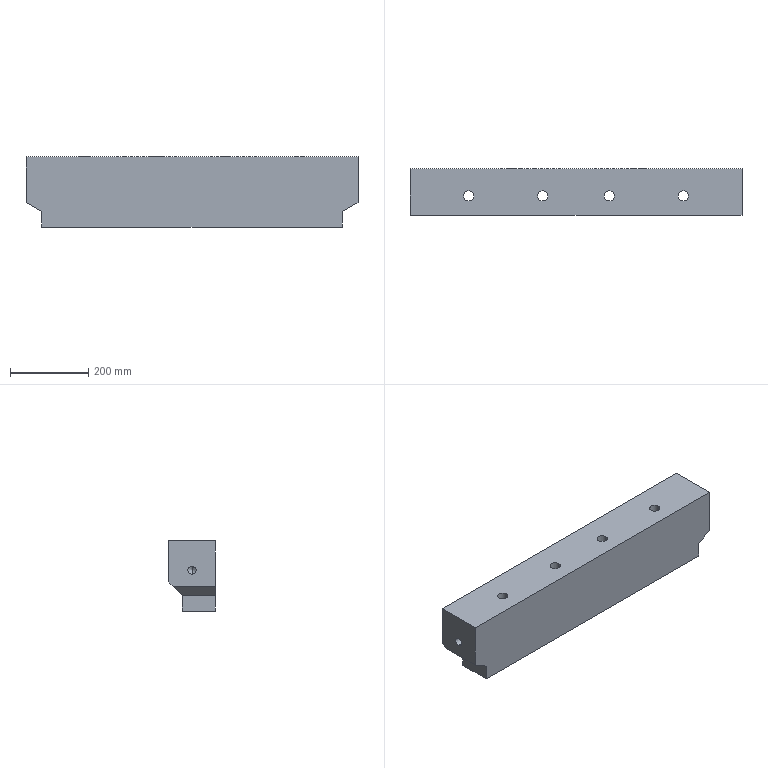Part | SolidWorks | features BaseBody 1 | 1 solid | 58 faces | box 850 x 120 x 180 mm | volume 15664153 mm3 | plane 26 | cylinder 20 | cone 12 | commonest cylinder face diameters 26 x8 17.5 x4 21 x4 38 x4